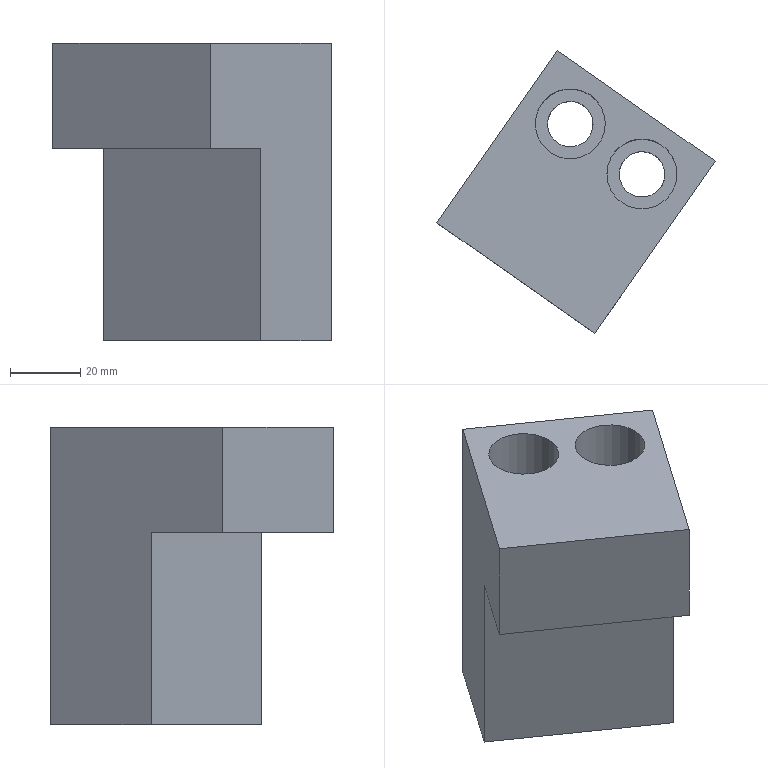Part | NX | features solid 2 | 1 solid | 14 faces | box 79.468 x 80.696 x 85 mm | volume 162358 mm3 | plane 9 | cylinder 4 | spline 1 | commonest cylinder face diameters 13 x2 20 x2
STEP:
#1=CARTESIAN_POINT('',(301.621,356.463,-125.));
#2=VERTEX_POINT('',#1);
#3=CARTESIAN_POINT('',(256.568,388.01,-125.));
#4=VERTEX_POINT('',#3);
#5=CARTESIAN_POINT('',(791.825,13.218,-125.));
#6=DIRECTION('',(-0.8192,0.5736,0.));
#7=VECTOR('',#6,1000.);
#8=LINE('',#5,#7);
#9=EDGE_CURVE('',#2,#4,#8,.T.);
#10=ORIENTED_EDGE('',*,*,#9,.F.);
#11=CARTESIAN_POINT('',(287.282,335.984,-125.));
#12=VERTEX_POINT('',#11);
#13=CARTESIAN_POINT('',(281.546,327.793,-125.));
#14=DIRECTION('',(-0.5736,-0.8192,0.));
#15=VECTOR('',#14,1000.);
#16=LINE('',#13,#15);
#17=EDGE_CURVE('',#12,#2,#16,.F.);
#18=ORIENTED_EDGE('',*,*,#17,.F.);
#19=CARTESIAN_POINT('',(242.228,367.531,-125.));
#20=VERTEX_POINT('',#19);
#21=CARTESIAN_POINT('',(283.186,338.852,-125.));
#22=DIRECTION('',(0.8192,-0.5736,0.));
#23=VECTOR('',#22,1000.);
#24=LINE('',#21,#23);
#25=EDGE_CURVE('',#12,#20,#24,.F.);
#26=ORIENTED_EDGE('',*,*,#25,.T.);
#27=CARTESIAN_POINT('',(-24.693,-13.672,-125.));
#28=DIRECTION('',(-0.5736,-0.8192,0.));
#29=VECTOR('',#28,1000.);
#30=LINE('',#27,#29);
#31=EDGE_CURVE('',#20,#4,#30,.F.);
#32=ORIENTED_EDGE('',*,*,#31,.T.);
#33=EDGE_LOOP('',(#10,#18,#26,#32));
#34=FACE_BOUND('',#33,.T.);
#35=CARTESIAN_POINT('',(510.565,-388.463,-125.));
#36=DIRECTION('',(0.,0.,-1.));
#37=DIRECTION('',(-0.342,0.9397,0.));
#38=AXIS2_PLACEMENT_3D('',#35,#36,#37);
#39=PLANE('',#38);
#40=ADVANCED_FACE('',(#34),#39,.T.);
#41=ORIENTED_EDGE('',*,*,#25,.F.);
#42=CARTESIAN_POINT('',(287.282,335.984,-95.));
#43=VERTEX_POINT('',#42);
#44=CARTESIAN_POINT('',(287.282,335.984,-100.));
#45=DIRECTION('',(0.,0.,-1.));
#46=VECTOR('',#45,1000.);
#47=LINE('',#44,#46);
#48=EDGE_CURVE('',#43,#12,#47,.T.);
#49=ORIENTED_EDGE('',*,*,#48,.F.);
#50=CARTESIAN_POINT('',(242.228,367.531,-95.));
#51=VERTEX_POINT('',#50);
#52=CARTESIAN_POINT('',(777.486,-7.261,-95.));
#53=DIRECTION('',(0.8192,-0.5736,0.));
#54=VECTOR('',#53,1000.);
#55=LINE('',#52,#54);
#56=EDGE_CURVE('',#43,#51,#55,.F.);
#57=ORIENTED_EDGE('',*,*,#56,.T.);
#58=CARTESIAN_POINT('',(242.228,367.531,-100.));
#59=DIRECTION('',(0.,0.,-1.));
#60=VECTOR('',#59,1000.);
#61=LINE('',#58,#60);
#62=EDGE_CURVE('',#51,#20,#61,.T.);
#63=ORIENTED_EDGE('',*,*,#62,.T.);
#64=EDGE_LOOP('',(#41,#49,#57,#63));
#65=FACE_BOUND('',#64,.T.);
#66=CARTESIAN_POINT('',(283.186,338.852,-100.));
#67=DIRECTION('',(0.5736,0.8192,0.));
#68=DIRECTION('',(0.8192,-0.5736,0.));
#69=AXIS2_PLACEMENT_3D('',#66,#67,#68);
#70=PLANE('',#69);
#71=ADVANCED_FACE('',(#65),#70,.F.);
#72=ORIENTED_EDGE('',*,*,#31,.F.);
#73=ORIENTED_EDGE('',*,*,#62,.F.);
#74=CARTESIAN_POINT('',(276.643,416.68,-95.));
#75=VERTEX_POINT('',#74);
#76=CARTESIAN_POINT('',(-24.693,-13.672,-95.));
#77=DIRECTION('',(-0.5736,-0.8192,0.));
#78=VECTOR('',#77,1000.);
#79=LINE('',#76,#78);
#80=EDGE_CURVE('',#51,#75,#79,.F.);
#81=ORIENTED_EDGE('',*,*,#80,.T.);
#82=CARTESIAN_POINT('',(276.643,416.68,-180.));
#83=VERTEX_POINT('',#82);
#84=CARTESIAN_POINT('',(276.643,416.68,-100.));
#85=DIRECTION('',(0.,0.,-1.));
#86=VECTOR('',#85,1000.);
#87=LINE('',#84,#86);
#88=EDGE_CURVE('',#75,#83,#87,.T.);
#89=ORIENTED_EDGE('',*,*,#88,.T.);
#90=CARTESIAN_POINT('',(256.568,388.01,-180.));
#91=VERTEX_POINT('',#90);
#92=CARTESIAN_POINT('',(256.568,388.01,-180.));
#93=CARTESIAN_POINT('',(263.259,397.566,-180.));
#94=CARTESIAN_POINT('',(269.951,407.123,-180.));
#95=CARTESIAN_POINT('',(276.643,416.68,-180.));
#96=B_SPLINE_CURVE_WITH_KNOTS('',3,(#92,#93,#94,#95),.UNSPECIFIED.,.F.,.F.,(4,4),(0.,0.035),.UNSPECIFIED.);
#97=EDGE_CURVE('',#91,#83,#96,.T.);
#98=ORIENTED_EDGE('',*,*,#97,.F.);
#99=CARTESIAN_POINT('',(256.568,388.01,-175.));
#100=DIRECTION('',(0.,0.,-1.));
#101=VECTOR('',#100,1000.);
#102=LINE('',#99,#101);
#103=EDGE_CURVE('',#91,#4,#102,.F.);
#104=ORIENTED_EDGE('',*,*,#103,.T.);
#105=EDGE_LOOP('',(#72,#73,#81,#89,#98,#104));
#106=FACE_BOUND('',#105,.T.);
#107=CARTESIAN_POINT('',(-24.693,-13.672,-100.));
#108=DIRECTION('',(0.8192,-0.5736,0.));
#109=DIRECTION('',(-0.5736,-0.8192,0.));
#110=AXIS2_PLACEMENT_3D('',#107,#108,#109);
#111=PLANE('',#110);
#112=ADVANCED_FACE('',(#106),#111,.F.);
#113=CARTESIAN_POINT('',(321.696,385.133,-95.));
#114=VERTEX_POINT('',#113);
#115=CARTESIAN_POINT('',(321.696,385.133,-180.));
#116=VERTEX_POINT('',#115);
#117=CARTESIAN_POINT('',(321.696,385.133,-100.));
#118=DIRECTION('',(0.,0.,-1.));
#119=VECTOR('',#118,1000.);
#120=LINE('',#117,#119);
#121=EDGE_CURVE('',#114,#116,#120,.T.);
#122=ORIENTED_EDGE('',*,*,#121,.T.);
#123=CARTESIAN_POINT('',(321.696,385.133,-180.));
#124=CARTESIAN_POINT('',(306.678,395.649,-180.));
#125=CARTESIAN_POINT('',(291.661,406.164,-180.));
#126=CARTESIAN_POINT('',(276.643,416.68,-180.));
#127=B_SPLINE_CURVE_WITH_KNOTS('',3,(#123,#124,#125,#126),.UNSPECIFIED.,.F.,.F.,(4,4),(0.,0.055),.UNSPECIFIED.);
#128=EDGE_CURVE('',#116,#83,#127,.T.);
#129=ORIENTED_EDGE('',*,*,#128,.T.);
#130=ORIENTED_EDGE('',*,*,#88,.F.);
#131=CARTESIAN_POINT('',(811.9,41.889,-95.));
#132=DIRECTION('',(0.8192,-0.5736,0.));
#133=VECTOR('',#132,1000.);
#134=LINE('',#131,#133);
#135=EDGE_CURVE('',#114,#75,#134,.F.);
#136=ORIENTED_EDGE('',*,*,#135,.F.);
#137=EDGE_LOOP('',(#122,#129,#130,#136));
#138=FACE_BOUND('',#137,.T.);
#139=CARTESIAN_POINT('',(313.505,390.869,-15.));
#140=DIRECTION('',(0.5736,0.8192,0.));
#141=DIRECTION('',(0.8192,-0.5736,0.));
#142=AXIS2_PLACEMENT_3D('',#139,#140,#141);
#143=PLANE('',#142);
#144=ADVANCED_FACE('',(#138),#143,.T.);
#145=ORIENTED_EDGE('',*,*,#17,.T.);
#146=CARTESIAN_POINT('',(301.621,356.463,-180.));
#147=VERTEX_POINT('',#146);
#148=CARTESIAN_POINT('',(301.621,356.463,-175.));
#149=DIRECTION('',(0.,0.,-1.));
#150=VECTOR('',#149,1000.);
#151=LINE('',#148,#150);
#152=EDGE_CURVE('',#147,#2,#151,.F.);
#153=ORIENTED_EDGE('',*,*,#152,.F.);
#154=CARTESIAN_POINT('',(301.621,356.463,-180.));
#155=CARTESIAN_POINT('',(308.313,366.02,-180.));
#156=CARTESIAN_POINT('',(315.005,375.576,-180.));
#157=CARTESIAN_POINT('',(321.696,385.133,-180.));
#158=B_SPLINE_CURVE_WITH_KNOTS('',3,(#154,#155,#156,#157),.UNSPECIFIED.,.F.,.F.,(4,4),(0.,0.035),.UNSPECIFIED.);
#159=EDGE_CURVE('',#147,#116,#158,.T.);
#160=ORIENTED_EDGE('',*,*,#159,.T.);
#161=ORIENTED_EDGE('',*,*,#121,.F.);
#162=CARTESIAN_POINT('',(20.361,-45.219,-95.));
#163=DIRECTION('',(-0.5736,-0.8192,0.));
#164=VECTOR('',#163,1000.);
#165=LINE('',#162,#164);
#166=EDGE_CURVE('',#43,#114,#165,.F.);
#167=ORIENTED_EDGE('',*,*,#166,.F.);
#168=ORIENTED_EDGE('',*,*,#48,.T.);
#169=EDGE_LOOP('',(#145,#153,#160,#161,#167,#168));
#170=FACE_BOUND('',#169,.T.);
#171=CARTESIAN_POINT('',(281.546,327.793,-100.));
#172=DIRECTION('',(0.8192,-0.5736,0.));
#173=DIRECTION('',(-0.5736,-0.8192,0.));
#174=AXIS2_PLACEMENT_3D('',#171,#172,#173);
#175=PLANE('',#174);
#176=ADVANCED_FACE('',(#170),#175,.T.);
#177=CARTESIAN_POINT('',(290.805,381.45,-95.));
#178=VERTEX_POINT('',#177);
#179=CARTESIAN_POINT('',(300.805,381.45,-95.));
#180=DIRECTION('',(0.,0.,-1.));
#181=DIRECTION('',(-1.,0.,0.));
#182=AXIS2_PLACEMENT_3D('',#179,#180,#181);
#183=CIRCLE('',#182,10.);
#184=EDGE_CURVE('',#178,#178,#183,.T.);
#185=ORIENTED_EDGE('',*,*,#184,.T.);
#186=EDGE_LOOP('',(#185));
#187=FACE_BOUND('',#186,.T.);
#188=CARTESIAN_POINT('',(270.326,395.789,-95.));
#189=VERTEX_POINT('',#188);
#190=CARTESIAN_POINT('',(280.326,395.789,-95.));
#191=DIRECTION('',(0.,0.,-1.));
#192=DIRECTION('',(-1.,0.,0.));
#193=AXIS2_PLACEMENT_3D('',#190,#191,#192);
#194=CIRCLE('',#193,10.);
#195=EDGE_CURVE('',#189,#189,#194,.T.);
#196=ORIENTED_EDGE('',*,*,#195,.T.);
#197=EDGE_LOOP('',(#196));
#198=FACE_BOUND('',#197,.T.);
#199=ORIENTED_EDGE('',*,*,#56,.F.);
#200=ORIENTED_EDGE('',*,*,#166,.T.);
#201=ORIENTED_EDGE('',*,*,#135,.T.);
#202=ORIENTED_EDGE('',*,*,#80,.F.);
#203=EDGE_LOOP('',(#199,#200,#201,#202));
#204=FACE_BOUND('',#203,.T.);
#205=CARTESIAN_POINT('',(510.565,-388.463,-95.));
#206=DIRECTION('',(0.,0.,-1.));
#207=DIRECTION('',(-0.342,0.9397,0.));
#208=AXIS2_PLACEMENT_3D('',#205,#206,#207);
#209=PLANE('',#208);
#210=ADVANCED_FACE('',(#187,#198,#204),#209,.F.);
#211=CARTESIAN_POINT('',(273.826,395.789,-150.));
#212=VERTEX_POINT('',#211);
#213=CARTESIAN_POINT('',(280.326,395.789,-150.));
#214=DIRECTION('',(0.,0.,-1.));
#215=DIRECTION('',(-1.,0.,0.));
#216=AXIS2_PLACEMENT_3D('',#213,#214,#215);
#217=CIRCLE('',#216,6.5);
#218=EDGE_CURVE('',#212,#212,#217,.T.);
#219=ORIENTED_EDGE('',*,*,#218,.F.);
#220=EDGE_LOOP('',(#219));
#221=FACE_BOUND('',#220,.T.);
#222=CARTESIAN_POINT('',(282.55,389.681,-180.));
#223=VERTEX_POINT('',#222);
#224=CARTESIAN_POINT('',(286.859,392.75,-180.));
#225=CARTESIAN_POINT('',(282.789,389.018,-180.));
#226=CARTESIAN_POINT('',(277.281,389.263,-180.));
#227=CARTESIAN_POINT('',(273.56,393.321,-180.));
#228=CARTESIAN_POINT('',(273.795,398.83,-180.));
#229=CARTESIAN_POINT('',(277.862,402.557,-180.));
#230=CARTESIAN_POINT('',(283.363,402.32,-180.));
#231=CARTESIAN_POINT('',(287.093,398.26,-180.));
#232=CARTESIAN_POINT('',(286.859,392.75,-180.));
#233=CARTESIAN_POINT('',(282.789,389.018,-180.));
#234=CARTESIAN_POINT('',(277.281,389.263,-180.));
#235=B_SPLINE_CURVE_WITH_KNOTS('',3,(#224,#225,#226,#227,#228,#229,#230,#231,#232,#233,#234),.UNSPECIFIED.,.T.,.F.,(1,1,1,1,1,1,1,1,1,1,1,1,1,1,1),(-0.01524,-0.01016,-0.00508,0.,0.00508,0.01016,0.01524,0.02032,0.0254,0.03048,0.03556,0.04064,0.04572,0.0508,0.05588),.UNSPECIFIED.);
#236=EDGE_CURVE('',#223,#223,#235,.T.);
#237=ORIENTED_EDGE('',*,*,#236,.T.);
#238=EDGE_LOOP('',(#237));
#239=FACE_BOUND('',#238,.T.);
#240=CARTESIAN_POINT('',(280.326,395.789,-145.));
#241=DIRECTION('',(0.,0.,1.));
#242=DIRECTION('',(0.342,-0.9397,0.));
#243=AXIS2_PLACEMENT_3D('',#240,#241,#242);
#244=CYLINDRICAL_SURFACE('',#243,6.5);
#245=ADVANCED_FACE('',(#221,#239),#244,.F.);
#246=ORIENTED_EDGE('',*,*,#218,.T.);
#247=EDGE_LOOP('',(#246));
#248=FACE_BOUND('',#247,.T.);
#249=CARTESIAN_POINT('',(270.326,395.789,-150.));
#250=VERTEX_POINT('',#249);
#251=CARTESIAN_POINT('',(280.326,395.789,-150.));
#252=DIRECTION('',(0.,0.,-1.));
#253=DIRECTION('',(-1.,0.,0.));
#254=AXIS2_PLACEMENT_3D('',#251,#252,#253);
#255=CIRCLE('',#254,10.);
#256=EDGE_CURVE('',#250,#250,#255,.T.);
#257=ORIENTED_EDGE('',*,*,#256,.F.);
#258=EDGE_LOOP('',(#257));
#259=FACE_BOUND('',#258,.T.);
#260=CARTESIAN_POINT('',(280.326,395.789,-150.));
#261=DIRECTION('',(0.,0.,-1.));
#262=DIRECTION('',(-0.342,0.9397,0.));
#263=AXIS2_PLACEMENT_3D('',#260,#261,#262);
#264=PLANE('',#263);
#265=ADVANCED_FACE('',(#248,#259),#264,.F.);
#266=ORIENTED_EDGE('',*,*,#195,.F.);
#267=EDGE_LOOP('',(#266));
#268=FACE_BOUND('',#267,.T.);
#269=ORIENTED_EDGE('',*,*,#256,.T.);
#270=EDGE_LOOP('',(#269));
#271=FACE_BOUND('',#270,.T.);
#272=CARTESIAN_POINT('',(280.326,395.789,-105.));
#273=DIRECTION('',(0.,0.,1.));
#274=DIRECTION('',(0.342,-0.9397,0.));
#275=AXIS2_PLACEMENT_3D('',#272,#273,#274);
#276=CYLINDRICAL_SURFACE('',#275,10.);
#277=ADVANCED_FACE('',(#268,#271),#276,.F.);
#278=CARTESIAN_POINT('',(294.305,381.45,-150.));
#279=VERTEX_POINT('',#278);
#280=CARTESIAN_POINT('',(300.805,381.45,-150.));
#281=DIRECTION('',(0.,0.,-1.));
#282=DIRECTION('',(-1.,0.,0.));
#283=AXIS2_PLACEMENT_3D('',#280,#281,#282);
#284=CIRCLE('',#283,6.5);
#285=EDGE_CURVE('',#279,#279,#284,.T.);
#286=ORIENTED_EDGE('',*,*,#285,.F.);
#287=EDGE_LOOP('',(#286));
#288=FACE_BOUND('',#287,.T.);
#289=CARTESIAN_POINT('',(303.028,375.342,-180.));
#290=VERTEX_POINT('',#289);
#291=CARTESIAN_POINT('',(307.338,378.411,-180.));
#292=CARTESIAN_POINT('',(303.268,374.679,-180.));
#293=CARTESIAN_POINT('',(297.76,374.923,-180.));
#294=CARTESIAN_POINT('',(294.039,378.981,-180.));
#295=CARTESIAN_POINT('',(294.274,384.491,-180.));
#296=CARTESIAN_POINT('',(298.341,388.217,-180.));
#297=CARTESIAN_POINT('',(303.842,387.98,-180.));
#298=CARTESIAN_POINT('',(307.572,383.921,-180.));
#299=CARTESIAN_POINT('',(307.338,378.411,-180.));
#300=CARTESIAN_POINT('',(303.268,374.679,-180.));
#301=CARTESIAN_POINT('',(297.76,374.923,-180.));
#302=B_SPLINE_CURVE_WITH_KNOTS('',3,(#291,#292,#293,#294,#295,#296,#297,#298,#299,#300,#301),.UNSPECIFIED.,.T.,.F.,(1,1,1,1,1,1,1,1,1,1,1,1,1,1,1),(-0.01524,-0.01016,-0.00508,0.,0.00508,0.01016,0.01524,0.02032,0.0254,0.03048,0.03556,0.04064,0.04572,0.0508,0.05588),.UNSPECIFIED.);
#303=EDGE_CURVE('',#290,#290,#302,.T.);
#304=ORIENTED_EDGE('',*,*,#303,.T.);
#305=EDGE_LOOP('',(#304));
#306=FACE_BOUND('',#305,.T.);
#307=CARTESIAN_POINT('',(300.805,381.45,-145.));
#308=DIRECTION('',(0.,0.,1.));
#309=DIRECTION('',(0.342,-0.9397,0.));
#310=AXIS2_PLACEMENT_3D('',#307,#308,#309);
#311=CYLINDRICAL_SURFACE('',#310,6.5);
#312=ADVANCED_FACE('',(#288,#306),#311,.F.);
#313=ORIENTED_EDGE('',*,*,#285,.T.);
#314=EDGE_LOOP('',(#313));
#315=FACE_BOUND('',#314,.T.);
#316=CARTESIAN_POINT('',(290.805,381.45,-150.));
#317=VERTEX_POINT('',#316);
#318=CARTESIAN_POINT('',(300.805,381.45,-150.));
#319=DIRECTION('',(0.,0.,-1.));
#320=DIRECTION('',(-1.,0.,0.));
#321=AXIS2_PLACEMENT_3D('',#318,#319,#320);
#322=CIRCLE('',#321,10.);
#323=EDGE_CURVE('',#317,#317,#322,.T.);
#324=ORIENTED_EDGE('',*,*,#323,.F.);
#325=EDGE_LOOP('',(#324));
#326=FACE_BOUND('',#325,.T.);
#327=CARTESIAN_POINT('',(300.805,381.45,-150.));
#328=DIRECTION('',(0.,0.,-1.));
#329=DIRECTION('',(-0.342,0.9397,0.));
#330=AXIS2_PLACEMENT_3D('',#327,#328,#329);
#331=PLANE('',#330);
#332=ADVANCED_FACE('',(#315,#326),#331,.F.);
#333=ORIENTED_EDGE('',*,*,#184,.F.);
#334=EDGE_LOOP('',(#333));
#335=FACE_BOUND('',#334,.T.);
#336=ORIENTED_EDGE('',*,*,#323,.T.);
#337=EDGE_LOOP('',(#336));
#338=FACE_BOUND('',#337,.T.);
#339=CARTESIAN_POINT('',(300.805,381.45,-105.));
#340=DIRECTION('',(0.,0.,1.));
#341=DIRECTION('',(0.342,-0.9397,0.));
#342=AXIS2_PLACEMENT_3D('',#339,#340,#341);
#343=CYLINDRICAL_SURFACE('',#342,10.);
#344=ADVANCED_FACE('',(#335,#338),#343,.F.);
#345=ORIENTED_EDGE('',*,*,#9,.T.);
#346=ORIENTED_EDGE('',*,*,#103,.F.);
#347=CARTESIAN_POINT('',(301.621,356.463,-180.));
#348=CARTESIAN_POINT('',(286.603,366.978,-180.));
#349=CARTESIAN_POINT('',(271.585,377.494,-180.));
#350=CARTESIAN_POINT('',(256.568,388.01,-180.));
#351=B_SPLINE_CURVE_WITH_KNOTS('',3,(#347,#348,#349,#350),.UNSPECIFIED.,.F.,.F.,(4,4),(0.,0.055),.UNSPECIFIED.);
#352=EDGE_CURVE('',#147,#91,#351,.T.);
#353=ORIENTED_EDGE('',*,*,#352,.F.);
#354=ORIENTED_EDGE('',*,*,#152,.T.);
#355=EDGE_LOOP('',(#345,#346,#353,#354));
#356=FACE_BOUND('',#355,.T.);
#357=CARTESIAN_POINT('',(289.334,365.066,-15.));
#358=DIRECTION('',(-0.5736,-0.8192,0.));
#359=DIRECTION('',(0.8192,-0.5736,0.));
#360=AXIS2_PLACEMENT_3D('',#357,#358,#359);
#361=PLANE('',#360);
#362=ADVANCED_FACE('',(#356),#361,.T.);
#363=ORIENTED_EDGE('',*,*,#303,.F.);
#364=EDGE_LOOP('',(#363));
#365=FACE_BOUND('',#364,.T.);
#366=ORIENTED_EDGE('',*,*,#236,.F.);
#367=EDGE_LOOP('',(#366));
#368=FACE_BOUND('',#367,.T.);
#369=ORIENTED_EDGE('',*,*,#352,.T.);
#370=ORIENTED_EDGE('',*,*,#97,.T.);
#371=ORIENTED_EDGE('',*,*,#128,.F.);
#372=ORIENTED_EDGE('',*,*,#159,.F.);
#373=EDGE_LOOP('',(#369,#370,#371,#372));
#374=FACE_BOUND('',#373,.T.);
#375=CARTESIAN_POINT('',(322.087,356.102,-180.));
#376=CARTESIAN_POINT('',(256.177,356.102,-180.));
#377=CARTESIAN_POINT('',(322.087,357.401,-180.));
#378=CARTESIAN_POINT('',(256.177,357.401,-180.));
#379=CARTESIAN_POINT('',(322.087,358.701,-180.));
#380=CARTESIAN_POINT('',(256.177,358.701,-180.));
#381=CARTESIAN_POINT('',(322.087,360.,-180.));
#382=CARTESIAN_POINT('',(256.177,360.,-180.));
#383=CARTESIAN_POINT('',(322.087,379.014,-180.));
#384=CARTESIAN_POINT('',(256.177,379.014,-180.));
#385=CARTESIAN_POINT('',(322.087,398.027,-180.));
#386=CARTESIAN_POINT('',(256.177,398.027,-180.));
#387=CARTESIAN_POINT('',(322.087,417.041,-180.));
#388=CARTESIAN_POINT('',(256.177,417.041,-180.));
#389=B_SPLINE_SURFACE_WITH_KNOTS('',3,1,((#375,#376),(#377,#378),(#379,#380),(#381,#382),(#383,#384),(#385,#386),(#387,#388)),.SURF_OF_LINEAR_EXTRUSION.,.F.,.F.,.F.,(4,3,4),(2,2),(-0.008475,0.,0.124),(0.,1.),.PIECEWISE_BEZIER_KNOTS.);
#390=ADVANCED_FACE('',(#365,#368,#374),#389,.F.);
#391=CLOSED_SHELL('',(#40,#71,#112,#144,#176,#210,#245,#265,#277,#312,#332,#344,#362,#390));
#392=MANIFOLD_SOLID_BREP('',#391);
#393=(LENGTH_UNIT()NAMED_UNIT(*)SI_UNIT(.MILLI.,.METRE.));
#394=UNCERTAINTY_MEASURE_WITH_UNIT(LENGTH_MEASURE(0.0508),#393,'','');
#395=(NAMED_UNIT(*)PLANE_ANGLE_UNIT()SI_UNIT($,.RADIAN.));
#396=(NAMED_UNIT(*)SI_UNIT($,.STERADIAN.)SOLID_ANGLE_UNIT());
#397=(GEOMETRIC_REPRESENTATION_CONTEXT(3)GLOBAL_UNCERTAINTY_ASSIGNED_CONTEXT((#394))GLOBAL_UNIT_ASSIGNED_CONTEXT((#393,#395,#396))REPRESENTATION_CONTEXT('',''));
#398=ADVANCED_BREP_SHAPE_REPRESENTATION('',(#392),#397);